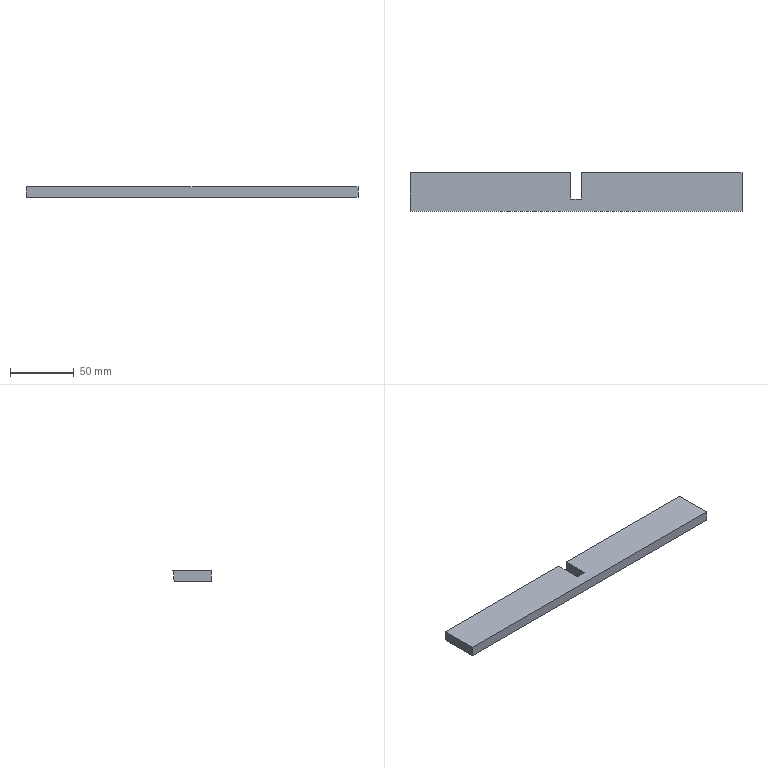Part | SolidWorks | features BaseBody 1 | 1 solid | 10 faces | box 260.4 x 30 x 8 mm | volume 60043 mm3 | plane 10
STEP:
#1=CARTESIAN_POINT('',(4.,15.,8.));
#2=VERTEX_POINT('',#1);
#3=CARTESIAN_POINT('',(4.,13.904,0.));
#4=VERTEX_POINT('',#3);
#5=CARTESIAN_POINT('',(4.,14.452,4.));
#6=DIRECTION('',(0.,-0.1357,-0.9907));
#7=VECTOR('',#6,1000.);
#8=LINE('',#5,#7);
#9=EDGE_CURVE('',#2,#4,#8,.T.);
#10=ORIENTED_EDGE('',*,*,#9,.F.);
#11=CARTESIAN_POINT('',(130.2,15.,8.));
#12=VERTEX_POINT('',#11);
#13=CARTESIAN_POINT('',(67.1,15.,8.));
#14=DIRECTION('',(-1.,0.,0.));
#15=VECTOR('',#14,1000.);
#16=LINE('',#13,#15);
#17=EDGE_CURVE('',#12,#2,#16,.T.);
#18=ORIENTED_EDGE('',*,*,#17,.F.);
#19=CARTESIAN_POINT('',(130.2,13.904,0.));
#20=VERTEX_POINT('',#19);
#21=CARTESIAN_POINT('',(130.2,14.452,4.));
#22=DIRECTION('',(0.,0.1357,0.9907));
#23=VECTOR('',#22,1000.);
#24=LINE('',#21,#23);
#25=EDGE_CURVE('',#20,#12,#24,.T.);
#26=ORIENTED_EDGE('',*,*,#25,.F.);
#27=CARTESIAN_POINT('',(67.1,13.904,0.));
#28=DIRECTION('',(1.,0.,0.));
#29=VECTOR('',#28,1000.);
#30=LINE('',#27,#29);
#31=EDGE_CURVE('',#4,#20,#30,.T.);
#32=ORIENTED_EDGE('',*,*,#31,.F.);
#33=EDGE_LOOP('',(#10,#18,#26,#32));
#34=FACE_OUTER_BOUND('',#33,.T.);
#35=CARTESIAN_POINT('',(4.,15.,8.));
#36=DIRECTION('',(0.,-0.9907,0.1357));
#37=DIRECTION('',(0.,-0.1357,-0.9907));
#38=AXIS2_PLACEMENT_3D('',#35,#36,#37);
#39=PLANE('',#38);
#40=ADVANCED_FACE('',(#34),#39,.F.);
#41=CARTESIAN_POINT('',(-4.,13.904,0.));
#42=VERTEX_POINT('',#41);
#43=CARTESIAN_POINT('',(-4.,-6.596,0.));
#44=VERTEX_POINT('',#43);
#45=CARTESIAN_POINT('',(-4.,-0.5479,0.));
#46=DIRECTION('',(0.,-1.,0.));
#47=VECTOR('',#46,1000.);
#48=LINE('',#45,#47);
#49=EDGE_CURVE('',#42,#44,#48,.T.);
#50=ORIENTED_EDGE('',*,*,#49,.T.);
#51=CARTESIAN_POINT('',(4.,-6.596,0.));
#52=VERTEX_POINT('',#51);
#53=CARTESIAN_POINT('',(0.,-6.596,0.));
#54=DIRECTION('',(1.,0.,0.));
#55=VECTOR('',#54,1000.);
#56=LINE('',#53,#55);
#57=EDGE_CURVE('',#44,#52,#56,.T.);
#58=ORIENTED_EDGE('',*,*,#57,.T.);
#59=CARTESIAN_POINT('',(4.,-0.5479,0.));
#60=DIRECTION('',(0.,1.,0.));
#61=VECTOR('',#60,1000.);
#62=LINE('',#59,#61);
#63=EDGE_CURVE('',#52,#4,#62,.T.);
#64=ORIENTED_EDGE('',*,*,#63,.T.);
#65=ORIENTED_EDGE('',*,*,#31,.T.);
#66=CARTESIAN_POINT('',(130.2,-15.,0.));
#67=VERTEX_POINT('',#66);
#68=CARTESIAN_POINT('',(130.2,-0.5479,0.));
#69=DIRECTION('',(0.,-1.,0.));
#70=VECTOR('',#69,1000.);
#71=LINE('',#68,#70);
#72=EDGE_CURVE('',#20,#67,#71,.T.);
#73=ORIENTED_EDGE('',*,*,#72,.T.);
#74=CARTESIAN_POINT('',(-130.2,-15.,0.));
#75=VERTEX_POINT('',#74);
#76=CARTESIAN_POINT('',(0.,-15.,0.));
#77=DIRECTION('',(-1.,0.,0.));
#78=VECTOR('',#77,1000.);
#79=LINE('',#76,#78);
#80=EDGE_CURVE('',#67,#75,#79,.T.);
#81=ORIENTED_EDGE('',*,*,#80,.T.);
#82=CARTESIAN_POINT('',(-130.2,13.904,0.));
#83=VERTEX_POINT('',#82);
#84=CARTESIAN_POINT('',(-130.2,-0.5479,0.));
#85=DIRECTION('',(0.,1.,0.));
#86=VECTOR('',#85,1000.);
#87=LINE('',#84,#86);
#88=EDGE_CURVE('',#75,#83,#87,.T.);
#89=ORIENTED_EDGE('',*,*,#88,.T.);
#90=CARTESIAN_POINT('',(0.,13.904,0.));
#91=DIRECTION('',(1.,0.,0.));
#92=VECTOR('',#91,1000.);
#93=LINE('',#90,#92);
#94=EDGE_CURVE('',#83,#42,#93,.T.);
#95=ORIENTED_EDGE('',*,*,#94,.T.);
#96=EDGE_LOOP('',(#50,#58,#64,#65,#73,#81,#89,#95));
#97=FACE_OUTER_BOUND('',#96,.T.);
#98=CARTESIAN_POINT('',(130.2,-15.,0.));
#99=DIRECTION('',(0.,0.,-1.));
#100=DIRECTION('',(-1.,0.,0.));
#101=AXIS2_PLACEMENT_3D('',#98,#99,#100);
#102=PLANE('',#101);
#103=ADVANCED_FACE('',(#97),#102,.T.);
#104=CARTESIAN_POINT('',(4.,-5.5,8.));
#105=VERTEX_POINT('',#104);
#106=CARTESIAN_POINT('',(4.,-5.5,8.));
#107=DIRECTION('',(0.,-0.1357,-0.9907));
#108=VECTOR('',#107,1000.);
#109=LINE('',#106,#108);
#110=EDGE_CURVE('',#105,#52,#109,.T.);
#111=ORIENTED_EDGE('',*,*,#110,.F.);
#112=CARTESIAN_POINT('',(4.,4.202,8.));
#113=DIRECTION('',(0.,-1.,0.));
#114=VECTOR('',#113,1000.);
#115=LINE('',#112,#114);
#116=EDGE_CURVE('',#2,#105,#115,.T.);
#117=ORIENTED_EDGE('',*,*,#116,.F.);
#118=ORIENTED_EDGE('',*,*,#9,.T.);
#119=ORIENTED_EDGE('',*,*,#63,.F.);
#120=EDGE_LOOP('',(#111,#117,#118,#119));
#121=FACE_OUTER_BOUND('',#120,.T.);
#122=CARTESIAN_POINT('',(4.,-6.725,8.));
#123=DIRECTION('',(1.,0.,0.));
#124=DIRECTION('',(0.,0.,-1.));
#125=AXIS2_PLACEMENT_3D('',#122,#123,#124);
#126=PLANE('',#125);
#127=ADVANCED_FACE('',(#121),#126,.F.);
#128=ORIENTED_EDGE('',*,*,#116,.T.);
#129=CARTESIAN_POINT('',(-4.,-5.5,8.));
#130=VERTEX_POINT('',#129);
#131=CARTESIAN_POINT('',(0.,-5.5,8.));
#132=DIRECTION('',(1.,0.,0.));
#133=VECTOR('',#132,1000.);
#134=LINE('',#131,#133);
#135=EDGE_CURVE('',#130,#105,#134,.T.);
#136=ORIENTED_EDGE('',*,*,#135,.F.);
#137=CARTESIAN_POINT('',(-4.,15.,8.));
#138=VERTEX_POINT('',#137);
#139=CARTESIAN_POINT('',(-4.,0.,8.));
#140=DIRECTION('',(0.,-1.,0.));
#141=VECTOR('',#140,1000.);
#142=LINE('',#139,#141);
#143=EDGE_CURVE('',#138,#130,#142,.T.);
#144=ORIENTED_EDGE('',*,*,#143,.F.);
#145=CARTESIAN_POINT('',(-130.2,15.,8.));
#146=VERTEX_POINT('',#145);
#147=CARTESIAN_POINT('',(0.,15.,8.));
#148=DIRECTION('',(1.,0.,0.));
#149=VECTOR('',#148,1000.);
#150=LINE('',#147,#149);
#151=EDGE_CURVE('',#146,#138,#150,.T.);
#152=ORIENTED_EDGE('',*,*,#151,.F.);
#153=CARTESIAN_POINT('',(-130.2,-15.,8.));
#154=VERTEX_POINT('',#153);
#155=CARTESIAN_POINT('',(-130.2,0.,8.));
#156=DIRECTION('',(0.,1.,0.));
#157=VECTOR('',#156,1000.);
#158=LINE('',#155,#157);
#159=EDGE_CURVE('',#154,#146,#158,.T.);
#160=ORIENTED_EDGE('',*,*,#159,.F.);
#161=CARTESIAN_POINT('',(130.2,-15.,8.));
#162=VERTEX_POINT('',#161);
#163=CARTESIAN_POINT('',(0.,-15.,8.));
#164=DIRECTION('',(-1.,0.,0.));
#165=VECTOR('',#164,1000.);
#166=LINE('',#163,#165);
#167=EDGE_CURVE('',#162,#154,#166,.T.);
#168=ORIENTED_EDGE('',*,*,#167,.F.);
#169=CARTESIAN_POINT('',(130.2,0.,8.));
#170=DIRECTION('',(0.,-1.,0.));
#171=VECTOR('',#170,1000.);
#172=LINE('',#169,#171);
#173=EDGE_CURVE('',#12,#162,#172,.T.);
#174=ORIENTED_EDGE('',*,*,#173,.F.);
#175=ORIENTED_EDGE('',*,*,#17,.T.);
#176=EDGE_LOOP('',(#128,#136,#144,#152,#160,#168,#174,#175));
#177=FACE_OUTER_BOUND('',#176,.T.);
#178=CARTESIAN_POINT('',(130.2,-15.,8.));
#179=DIRECTION('',(0.,0.,-1.));
#180=DIRECTION('',(-1.,0.,0.));
#181=AXIS2_PLACEMENT_3D('',#178,#179,#180);
#182=PLANE('',#181);
#183=ADVANCED_FACE('',(#177),#182,.F.);
#184=ORIENTED_EDGE('',*,*,#25,.T.);
#185=ORIENTED_EDGE('',*,*,#173,.T.);
#186=CARTESIAN_POINT('',(130.2,-15.,4.));
#187=DIRECTION('',(0.,0.,1.));
#188=VECTOR('',#187,1000.);
#189=LINE('',#186,#188);
#190=EDGE_CURVE('',#67,#162,#189,.T.);
#191=ORIENTED_EDGE('',*,*,#190,.F.);
#192=ORIENTED_EDGE('',*,*,#72,.F.);
#193=EDGE_LOOP('',(#184,#185,#191,#192));
#194=FACE_OUTER_BOUND('',#193,.T.);
#195=CARTESIAN_POINT('',(130.2,-15.,0.));
#196=DIRECTION('',(-1.,0.,0.));
#197=DIRECTION('',(0.,0.,1.));
#198=AXIS2_PLACEMENT_3D('',#195,#196,#197);
#199=PLANE('',#198);
#200=ADVANCED_FACE('',(#194),#199,.F.);
#201=CARTESIAN_POINT('',(-4.,-6.048,4.));
#202=DIRECTION('',(0.,-0.1357,-0.9907));
#203=VECTOR('',#202,1000.);
#204=LINE('',#201,#203);
#205=EDGE_CURVE('',#130,#44,#204,.T.);
#206=ORIENTED_EDGE('',*,*,#205,.F.);
#207=ORIENTED_EDGE('',*,*,#135,.T.);
#208=ORIENTED_EDGE('',*,*,#110,.T.);
#209=ORIENTED_EDGE('',*,*,#57,.F.);
#210=EDGE_LOOP('',(#206,#207,#208,#209));
#211=FACE_OUTER_BOUND('',#210,.T.);
#212=CARTESIAN_POINT('',(-4.,-5.5,8.));
#213=DIRECTION('',(0.,-0.9907,0.1357));
#214=DIRECTION('',(0.,-0.1357,-0.9907));
#215=AXIS2_PLACEMENT_3D('',#212,#213,#214);
#216=PLANE('',#215);
#217=ADVANCED_FACE('',(#211),#216,.F.);
#218=CARTESIAN_POINT('',(-4.,15.,8.));
#219=DIRECTION('',(0.,-0.1357,-0.9907));
#220=VECTOR('',#219,1000.);
#221=LINE('',#218,#220);
#222=EDGE_CURVE('',#138,#42,#221,.T.);
#223=ORIENTED_EDGE('',*,*,#222,.F.);
#224=ORIENTED_EDGE('',*,*,#143,.T.);
#225=ORIENTED_EDGE('',*,*,#205,.T.);
#226=ORIENTED_EDGE('',*,*,#49,.F.);
#227=EDGE_LOOP('',(#223,#224,#225,#226));
#228=FACE_OUTER_BOUND('',#227,.T.);
#229=CARTESIAN_POINT('',(-4.,-6.725,0.));
#230=DIRECTION('',(-1.,0.,0.));
#231=DIRECTION('',(0.,0.,1.));
#232=AXIS2_PLACEMENT_3D('',#229,#230,#231);
#233=PLANE('',#232);
#234=ADVANCED_FACE('',(#228),#233,.F.);
#235=ORIENTED_EDGE('',*,*,#222,.T.);
#236=ORIENTED_EDGE('',*,*,#94,.F.);
#237=CARTESIAN_POINT('',(-130.2,14.452,4.));
#238=DIRECTION('',(0.,-0.1357,-0.9907));
#239=VECTOR('',#238,1000.);
#240=LINE('',#237,#239);
#241=EDGE_CURVE('',#146,#83,#240,.T.);
#242=ORIENTED_EDGE('',*,*,#241,.F.);
#243=ORIENTED_EDGE('',*,*,#151,.T.);
#244=EDGE_LOOP('',(#235,#236,#242,#243));
#245=FACE_OUTER_BOUND('',#244,.T.);
#246=CARTESIAN_POINT('',(-130.2,15.,8.));
#247=DIRECTION('',(0.,-0.9907,0.1357));
#248=DIRECTION('',(0.,-0.1357,-0.9907));
#249=AXIS2_PLACEMENT_3D('',#246,#247,#248);
#250=PLANE('',#249);
#251=ADVANCED_FACE('',(#245),#250,.F.);
#252=ORIENTED_EDGE('',*,*,#241,.T.);
#253=ORIENTED_EDGE('',*,*,#88,.F.);
#254=CARTESIAN_POINT('',(-130.2,-15.,4.));
#255=DIRECTION('',(0.,0.,-1.));
#256=VECTOR('',#255,1000.);
#257=LINE('',#254,#256);
#258=EDGE_CURVE('',#154,#75,#257,.T.);
#259=ORIENTED_EDGE('',*,*,#258,.F.);
#260=ORIENTED_EDGE('',*,*,#159,.T.);
#261=EDGE_LOOP('',(#252,#253,#259,#260));
#262=FACE_OUTER_BOUND('',#261,.T.);
#263=CARTESIAN_POINT('',(-130.2,-15.,8.));
#264=DIRECTION('',(1.,0.,0.));
#265=DIRECTION('',(0.,0.,-1.));
#266=AXIS2_PLACEMENT_3D('',#263,#264,#265);
#267=PLANE('',#266);
#268=ADVANCED_FACE('',(#262),#267,.F.);
#269=ORIENTED_EDGE('',*,*,#190,.T.);
#270=ORIENTED_EDGE('',*,*,#167,.T.);
#271=ORIENTED_EDGE('',*,*,#258,.T.);
#272=ORIENTED_EDGE('',*,*,#80,.F.);
#273=EDGE_LOOP('',(#269,#270,#271,#272));
#274=FACE_OUTER_BOUND('',#273,.T.);
#275=CARTESIAN_POINT('',(130.2,-15.,0.));
#276=DIRECTION('',(0.,1.,0.));
#277=DIRECTION('',(-1.,0.,0.));
#278=AXIS2_PLACEMENT_3D('',#275,#276,#277);
#279=PLANE('',#278);
#280=ADVANCED_FACE('',(#274),#279,.F.);
#281=CLOSED_SHELL('',(#40,#103,#127,#183,#200,#217,#234,#251,#268,#280));
#282=MANIFOLD_SOLID_BREP('',#281);
#283=CARTESIAN_POINT('',(0.,0.,0.));
#284=DIRECTION('',(0.,0.,1.));
#285=DIRECTION('',(1.,0.,0.));
#286=AXIS2_PLACEMENT_3D('',#283,#284,#285);
#287=(LENGTH_UNIT()NAMED_UNIT(*)SI_UNIT(.MILLI.,.METRE.));
#288=UNCERTAINTY_MEASURE_WITH_UNIT(LENGTH_MEASURE(0.00001),#287,'','');
#289=(NAMED_UNIT(*)PLANE_ANGLE_UNIT()SI_UNIT($,.RADIAN.));
#290=(NAMED_UNIT(*)SI_UNIT($,.STERADIAN.)SOLID_ANGLE_UNIT());
#291=(GEOMETRIC_REPRESENTATION_CONTEXT(3)GLOBAL_UNCERTAINTY_ASSIGNED_CONTEXT((#288))GLOBAL_UNIT_ASSIGNED_CONTEXT((#287,#289,#290))REPRESENTATION_CONTEXT('',''));
#292=ADVANCED_BREP_SHAPE_REPRESENTATION('',(#282,#286),#291);